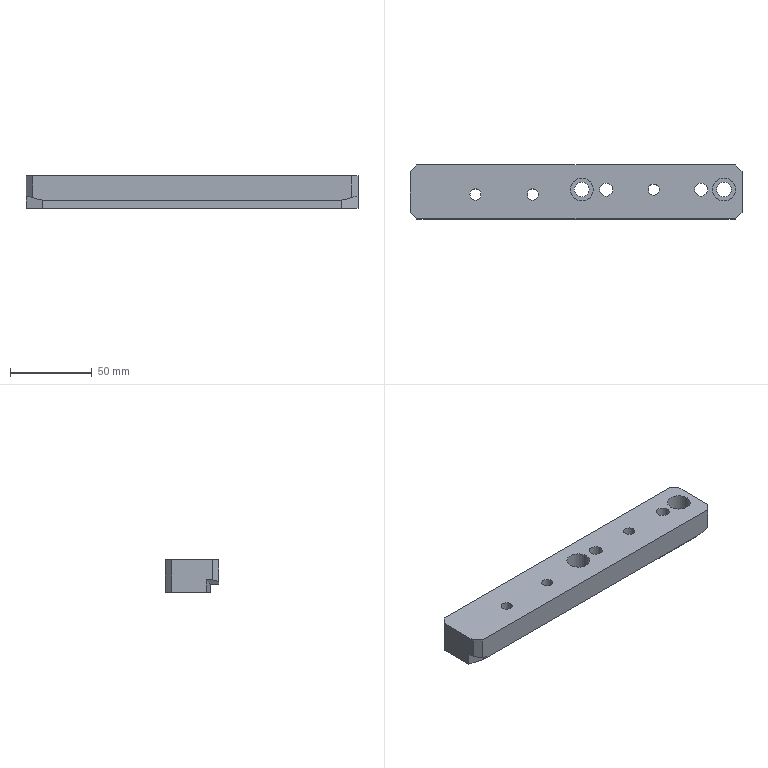Part | NX | features 20 2 | 1 solid | 27 faces | box 203 x 33 x 20 mm | volume 119525 mm3 | plane 18 | cylinder 9 | commonest cylinder face diameters 6.8 x3 8.001 x2 9 x2 14 x2
STEP:
#1=CARTESIAN_POINT('',(-35.998,435.5,16.5));
#2=VERTEX_POINT('',#1);
#3=CARTESIAN_POINT('',(-39.999,435.5,16.5));
#4=DIRECTION('',(0.,0.,1.));
#5=DIRECTION('',(1.,0.,0.));
#6=AXIS2_PLACEMENT_3D('',#3,#4,#5);
#7=CIRCLE('',#6,4.);
#8=EDGE_CURVE('',#2,#2,#7,.T.);
#9=ORIENTED_EDGE('',*,*,#8,.F.);
#10=EDGE_LOOP('',(#9));
#11=FACE_BOUND('',#10,.T.);
#12=CARTESIAN_POINT('',(22.002,435.5,16.5));
#13=VERTEX_POINT('',#12);
#14=CARTESIAN_POINT('',(18.001,435.5,16.5));
#15=DIRECTION('',(0.,0.,-1.));
#16=DIRECTION('',(1.,0.,0.));
#17=AXIS2_PLACEMENT_3D('',#14,#15,#16);
#18=CIRCLE('',#17,4.);
#19=EDGE_CURVE('',#13,#13,#18,.T.);
#20=ORIENTED_EDGE('',*,*,#19,.T.);
#21=EDGE_LOOP('',(#20));
#22=FACE_BOUND('',#21,.T.);
#23=CARTESIAN_POINT('',(39.001,435.5,16.5));
#24=VERTEX_POINT('',#23);
#25=CARTESIAN_POINT('',(32.001,435.5,16.5));
#26=DIRECTION('',(0.,0.,1.));
#27=DIRECTION('',(1.,0.,0.));
#28=AXIS2_PLACEMENT_3D('',#25,#26,#27);
#29=CIRCLE('',#28,7.);
#30=EDGE_CURVE('',#24,#24,#29,.T.);
#31=ORIENTED_EDGE('',*,*,#30,.F.);
#32=EDGE_LOOP('',(#31));
#33=FACE_BOUND('',#32,.T.);
#34=CARTESIAN_POINT('',(-155.999,417.5,16.5));
#35=VERTEX_POINT('',#34);
#36=CARTESIAN_POINT('',(39.001,417.5,16.5));
#37=VERTEX_POINT('',#36);
#38=CARTESIAN_POINT('',(-24.999,417.5,16.5));
#39=DIRECTION('',(1.,0.,0.));
#40=VECTOR('',#39,1000.);
#41=LINE('',#38,#40);
#42=EDGE_CURVE('',#35,#37,#41,.T.);
#43=ORIENTED_EDGE('',*,*,#42,.T.);
#44=CARTESIAN_POINT('',(43.001,421.5,16.5));
#45=VERTEX_POINT('',#44);
#46=CARTESIAN_POINT('',(39.001,417.5,16.5));
#47=DIRECTION('',(0.7071,0.7071,0.));
#48=VECTOR('',#47,1000.);
#49=LINE('',#46,#48);
#50=EDGE_CURVE('',#37,#45,#49,.T.);
#51=ORIENTED_EDGE('',*,*,#50,.T.);
#52=CARTESIAN_POINT('',(43.001,446.5,16.5));
#53=VERTEX_POINT('',#52);
#54=CARTESIAN_POINT('',(43.001,450.5,16.5));
#55=DIRECTION('',(0.,1.,0.));
#56=VECTOR('',#55,1000.);
#57=LINE('',#54,#56);
#58=EDGE_CURVE('',#45,#53,#57,.T.);
#59=ORIENTED_EDGE('',*,*,#58,.T.);
#60=CARTESIAN_POINT('',(39.001,450.5,16.5));
#61=VERTEX_POINT('',#60);
#62=CARTESIAN_POINT('',(43.001,446.5,16.5));
#63=DIRECTION('',(-0.7071,0.7071,0.));
#64=VECTOR('',#63,1000.);
#65=LINE('',#62,#64);
#66=EDGE_CURVE('',#53,#61,#65,.T.);
#67=ORIENTED_EDGE('',*,*,#66,.T.);
#68=CARTESIAN_POINT('',(-155.999,450.5,16.5));
#69=VERTEX_POINT('',#68);
#70=CARTESIAN_POINT('',(-104.999,450.5,16.5));
#71=DIRECTION('',(-1.,0.,0.));
#72=VECTOR('',#71,1000.);
#73=LINE('',#70,#72);
#74=EDGE_CURVE('',#61,#69,#73,.T.);
#75=ORIENTED_EDGE('',*,*,#74,.T.);
#76=CARTESIAN_POINT('',(-159.999,446.5,16.5));
#77=VERTEX_POINT('',#76);
#78=CARTESIAN_POINT('',(-155.999,450.5,16.5));
#79=DIRECTION('',(-0.7071,-0.7071,0.));
#80=VECTOR('',#79,1000.);
#81=LINE('',#78,#80);
#82=EDGE_CURVE('',#69,#77,#81,.T.);
#83=ORIENTED_EDGE('',*,*,#82,.T.);
#84=CARTESIAN_POINT('',(-159.999,421.5,16.5));
#85=VERTEX_POINT('',#84);
#86=CARTESIAN_POINT('',(-159.999,417.5,16.5));
#87=DIRECTION('',(0.,-1.,0.));
#88=VECTOR('',#87,1000.);
#89=LINE('',#86,#88);
#90=EDGE_CURVE('',#77,#85,#89,.T.);
#91=ORIENTED_EDGE('',*,*,#90,.T.);
#92=CARTESIAN_POINT('',(-159.999,421.5,16.5));
#93=DIRECTION('',(0.7071,-0.7071,0.));
#94=VECTOR('',#93,1000.);
#95=LINE('',#92,#94);
#96=EDGE_CURVE('',#85,#35,#95,.T.);
#97=ORIENTED_EDGE('',*,*,#96,.T.);
#98=EDGE_LOOP('',(#43,#51,#59,#67,#75,#83,#91,#97));
#99=FACE_BOUND('',#98,.T.);
#100=CARTESIAN_POINT('',(-81.599,432.45,16.5));
#101=VERTEX_POINT('',#100);
#102=CARTESIAN_POINT('',(-84.999,432.45,16.5));
#103=DIRECTION('',(0.,0.,1.));
#104=DIRECTION('',(1.,0.,0.));
#105=AXIS2_PLACEMENT_3D('',#102,#103,#104);
#106=CIRCLE('',#105,3.4);
#107=EDGE_CURVE('',#101,#101,#106,.T.);
#108=ORIENTED_EDGE('',*,*,#107,.F.);
#109=EDGE_LOOP('',(#108));
#110=FACE_BOUND('',#109,.T.);
#111=CARTESIAN_POINT('',(-116.599,432.45,16.5));
#112=VERTEX_POINT('',#111);
#113=CARTESIAN_POINT('',(-119.999,432.45,16.5));
#114=DIRECTION('',(0.,0.,1.));
#115=DIRECTION('',(1.,0.,0.));
#116=AXIS2_PLACEMENT_3D('',#113,#114,#115);
#117=CIRCLE('',#116,3.4);
#118=EDGE_CURVE('',#112,#112,#117,.T.);
#119=ORIENTED_EDGE('',*,*,#118,.F.);
#120=EDGE_LOOP('',(#119));
#121=FACE_BOUND('',#120,.T.);
#122=CARTESIAN_POINT('',(-47.999,435.5,16.5));
#123=VERTEX_POINT('',#122);
#124=CARTESIAN_POINT('',(-54.999,435.5,16.5));
#125=DIRECTION('',(0.,0.,1.));
#126=DIRECTION('',(1.,0.,0.));
#127=AXIS2_PLACEMENT_3D('',#124,#125,#126);
#128=CIRCLE('',#127,7.);
#129=EDGE_CURVE('',#123,#123,#128,.T.);
#130=ORIENTED_EDGE('',*,*,#129,.F.);
#131=EDGE_LOOP('',(#130));
#132=FACE_BOUND('',#131,.T.);
#133=CARTESIAN_POINT('',(-7.599,435.5,16.5));
#134=VERTEX_POINT('',#133);
#135=CARTESIAN_POINT('',(-10.999,435.5,16.5));
#136=DIRECTION('',(0.,0.,-1.));
#137=DIRECTION('',(1.,0.,0.));
#138=AXIS2_PLACEMENT_3D('',#135,#136,#137);
#139=CIRCLE('',#138,3.4);
#140=EDGE_CURVE('',#134,#134,#139,.T.);
#141=ORIENTED_EDGE('',*,*,#140,.T.);
#142=EDGE_LOOP('',(#141));
#143=FACE_BOUND('',#142,.T.);
#144=CARTESIAN_POINT('',(-24.999,450.5,16.5));
#145=DIRECTION('',(0.,0.,1.));
#146=DIRECTION('',(-1.,0.,0.));
#147=AXIS2_PLACEMENT_3D('',#144,#145,#146);
#148=PLANE('',#147);
#149=ADVANCED_FACE('',(#11,#22,#33,#99,#110,#121,#132,#143),#148,.T.);
#150=CARTESIAN_POINT('',(-35.998,435.5,-3.5));
#151=VERTEX_POINT('',#150);
#152=CARTESIAN_POINT('',(-39.999,435.5,-3.5));
#153=DIRECTION('',(0.,0.,1.));
#154=DIRECTION('',(1.,0.,0.));
#155=AXIS2_PLACEMENT_3D('',#152,#153,#154);
#156=CIRCLE('',#155,4.);
#157=EDGE_CURVE('',#151,#151,#156,.T.);
#158=ORIENTED_EDGE('',*,*,#157,.F.);
#159=EDGE_LOOP('',(#158));
#160=FACE_BOUND('',#159,.T.);
#161=ORIENTED_EDGE('',*,*,#8,.T.);
#162=EDGE_LOOP('',(#161));
#163=FACE_BOUND('',#162,.T.);
#164=CARTESIAN_POINT('',(-39.999,435.5,42.5));
#165=DIRECTION('',(0.,0.,-1.));
#166=DIRECTION('',(1.,0.,0.));
#167=AXIS2_PLACEMENT_3D('',#164,#165,#166);
#168=CYLINDRICAL_SURFACE('',#167,4.);
#169=ADVANCED_FACE('',(#160,#163),#168,.F.);
#170=CARTESIAN_POINT('',(22.002,435.5,-3.5));
#171=VERTEX_POINT('',#170);
#172=CARTESIAN_POINT('',(18.001,435.5,-3.5));
#173=DIRECTION('',(0.,0.,-1.));
#174=DIRECTION('',(1.,0.,0.));
#175=AXIS2_PLACEMENT_3D('',#172,#173,#174);
#176=CIRCLE('',#175,4.);
#177=EDGE_CURVE('',#171,#171,#176,.T.);
#178=ORIENTED_EDGE('',*,*,#177,.T.);
#179=EDGE_LOOP('',(#178));
#180=FACE_BOUND('',#179,.T.);
#181=ORIENTED_EDGE('',*,*,#19,.F.);
#182=EDGE_LOOP('',(#181));
#183=FACE_BOUND('',#182,.T.);
#184=CARTESIAN_POINT('',(18.001,435.5,42.5));
#185=DIRECTION('',(0.,0.,-1.));
#186=DIRECTION('',(1.,0.,0.));
#187=AXIS2_PLACEMENT_3D('',#184,#185,#186);
#188=CYLINDRICAL_SURFACE('',#187,4.);
#189=ADVANCED_FACE('',(#180,#183),#188,.F.);
#190=CARTESIAN_POINT('',(36.501,435.5,6.5));
#191=VERTEX_POINT('',#190);
#192=CARTESIAN_POINT('',(32.001,435.5,6.5));
#193=DIRECTION('',(0.,0.,-1.));
#194=DIRECTION('',(1.,0.,0.));
#195=AXIS2_PLACEMENT_3D('',#192,#193,#194);
#196=CIRCLE('',#195,4.5);
#197=EDGE_CURVE('',#191,#191,#196,.T.);
#198=ORIENTED_EDGE('',*,*,#197,.T.);
#199=EDGE_LOOP('',(#198));
#200=FACE_BOUND('',#199,.T.);
#201=CARTESIAN_POINT('',(39.001,435.5,6.5));
#202=VERTEX_POINT('',#201);
#203=CARTESIAN_POINT('',(32.001,435.5,6.5));
#204=DIRECTION('',(0.,0.,1.));
#205=DIRECTION('',(1.,0.,0.));
#206=AXIS2_PLACEMENT_3D('',#203,#204,#205);
#207=CIRCLE('',#206,7.);
#208=EDGE_CURVE('',#202,#202,#207,.T.);
#209=ORIENTED_EDGE('',*,*,#208,.T.);
#210=EDGE_LOOP('',(#209));
#211=FACE_BOUND('',#210,.T.);
#212=CARTESIAN_POINT('',(265.844,302.3,6.5));
#213=DIRECTION('',(0.,0.,1.));
#214=DIRECTION('',(0.,1.,0.));
#215=AXIS2_PLACEMENT_3D('',#212,#213,#214);
#216=PLANE('',#215);
#217=ADVANCED_FACE('',(#200,#211),#216,.T.);
#218=CARTESIAN_POINT('',(-159.999,425.179,4.179));
#219=VERTEX_POINT('',#218);
#220=CARTESIAN_POINT('',(-159.999,421.5,4.179));
#221=VERTEX_POINT('',#220);
#222=CARTESIAN_POINT('',(-159.999,425.179,4.179));
#223=DIRECTION('',(0.,-1.,0.));
#224=VECTOR('',#223,1000.);
#225=LINE('',#222,#224);
#226=EDGE_CURVE('',#219,#221,#225,.T.);
#227=ORIENTED_EDGE('',*,*,#226,.F.);
#228=CARTESIAN_POINT('',(-150.,422.5,1.5));
#229=VERTEX_POINT('',#228);
#230=CARTESIAN_POINT('',(-150.,422.5,1.5));
#231=DIRECTION('',(-0.9351,0.2506,0.2506));
#232=VECTOR('',#231,1000.);
#233=LINE('',#230,#232);
#234=EDGE_CURVE('',#229,#219,#233,.T.);
#235=ORIENTED_EDGE('',*,*,#234,.F.);
#236=CARTESIAN_POINT('',(-149.999,422.5,1.5));
#237=VERTEX_POINT('',#236);
#238=CARTESIAN_POINT('',(-94.02,422.5,-13.5));
#239=DIRECTION('',(-0.9659,0.,0.2588));
#240=VECTOR('',#239,1000.);
#241=LINE('',#238,#240);
#242=EDGE_CURVE('',#237,#229,#241,.T.);
#243=ORIENTED_EDGE('',*,*,#242,.F.);
#244=CARTESIAN_POINT('',(-149.999,417.5,1.5));
#245=VERTEX_POINT('',#244);
#246=CARTESIAN_POINT('',(-149.999,417.5,1.5));
#247=DIRECTION('',(0.,1.,0.));
#248=VECTOR('',#247,1000.);
#249=LINE('',#246,#248);
#250=EDGE_CURVE('',#245,#237,#249,.T.);
#251=ORIENTED_EDGE('',*,*,#250,.F.);
#252=CARTESIAN_POINT('',(-155.999,417.5,3.108));
#253=VERTEX_POINT('',#252);
#254=CARTESIAN_POINT('',(-149.999,417.5,1.5));
#255=DIRECTION('',(0.9659,0.,-0.2588));
#256=VECTOR('',#255,1000.);
#257=LINE('',#254,#256);
#258=EDGE_CURVE('',#253,#245,#257,.T.);
#259=ORIENTED_EDGE('',*,*,#258,.F.);
#260=CARTESIAN_POINT('',(-142.948,404.449,-0.3894));
#261=DIRECTION('',(-0.6947,0.6947,0.1862));
#262=VECTOR('',#261,1000.);
#263=LINE('',#260,#262);
#264=EDGE_CURVE('',#253,#221,#263,.T.);
#265=ORIENTED_EDGE('',*,*,#264,.T.);
#266=EDGE_LOOP('',(#227,#235,#243,#251,#259,#265));
#267=FACE_BOUND('',#266,.T.);
#268=CARTESIAN_POINT('',(-149.999,396.891,1.5));
#269=DIRECTION('',(-0.2588,0.,-0.9659));
#270=DIRECTION('',(0.9659,0.,-0.2588));
#271=AXIS2_PLACEMENT_3D('',#268,#269,#270);
#272=PLANE('',#271);
#273=ADVANCED_FACE('',(#267),#272,.T.);
#274=ORIENTED_EDGE('',*,*,#250,.T.);
#275=CARTESIAN_POINT('',(32.999,422.5,1.5));
#276=VERTEX_POINT('',#275);
#277=CARTESIAN_POINT('',(-35.001,422.5,1.5));
#278=DIRECTION('',(-1.,0.,0.));
#279=VECTOR('',#278,1000.);
#280=LINE('',#277,#279);
#281=EDGE_CURVE('',#276,#237,#280,.T.);
#282=ORIENTED_EDGE('',*,*,#281,.F.);
#283=CARTESIAN_POINT('',(33.001,422.5,1.5));
#284=VERTEX_POINT('',#283);
#285=CARTESIAN_POINT('',(43.001,425.18,1.5));
#286=DIRECTION('',(-0.9659,-0.2588,0.));
#287=VECTOR('',#286,1000.);
#288=LINE('',#285,#287);
#289=EDGE_CURVE('',#284,#276,#288,.T.);
#290=ORIENTED_EDGE('',*,*,#289,.F.);
#291=CARTESIAN_POINT('',(33.001,417.5,1.5));
#292=VERTEX_POINT('',#291);
#293=CARTESIAN_POINT('',(33.001,425.18,1.5));
#294=DIRECTION('',(0.,-1.,0.));
#295=VECTOR('',#294,1000.);
#296=LINE('',#293,#295);
#297=EDGE_CURVE('',#284,#292,#296,.T.);
#298=ORIENTED_EDGE('',*,*,#297,.T.);
#299=CARTESIAN_POINT('',(-24.999,417.5,1.5));
#300=DIRECTION('',(-1.,0.,0.));
#301=VECTOR('',#300,1000.);
#302=LINE('',#299,#301);
#303=EDGE_CURVE('',#292,#245,#302,.T.);
#304=ORIENTED_EDGE('',*,*,#303,.T.);
#305=EDGE_LOOP('',(#274,#282,#290,#298,#304));
#306=FACE_BOUND('',#305,.T.);
#307=CARTESIAN_POINT('',(-2.728,396.891,1.5));
#308=DIRECTION('',(0.,0.,-1.));
#309=DIRECTION('',(1.,0.,0.));
#310=AXIS2_PLACEMENT_3D('',#307,#308,#309);
#311=PLANE('',#310);
#312=ADVANCED_FACE('',(#306),#311,.T.);
#313=CARTESIAN_POINT('',(39.001,417.5,3.108));
#314=VERTEX_POINT('',#313);
#315=CARTESIAN_POINT('',(33.001,417.5,1.5));
#316=DIRECTION('',(0.9659,0.,0.2588));
#317=VECTOR('',#316,1000.);
#318=LINE('',#315,#317);
#319=EDGE_CURVE('',#292,#314,#318,.T.);
#320=ORIENTED_EDGE('',*,*,#319,.F.);
#321=ORIENTED_EDGE('',*,*,#297,.F.);
#322=CARTESIAN_POINT('',(43.001,425.18,4.179));
#323=VERTEX_POINT('',#322);
#324=CARTESIAN_POINT('',(42.373,425.012,4.011));
#325=DIRECTION('',(-0.9351,-0.2506,-0.2506));
#326=VECTOR('',#325,1000.);
#327=LINE('',#324,#326);
#328=EDGE_CURVE('',#323,#284,#327,.T.);
#329=ORIENTED_EDGE('',*,*,#328,.F.);
#330=CARTESIAN_POINT('',(43.001,421.5,4.179));
#331=VERTEX_POINT('',#330);
#332=CARTESIAN_POINT('',(43.001,417.5,4.179));
#333=DIRECTION('',(0.,1.,0.));
#334=VECTOR('',#333,1000.);
#335=LINE('',#332,#334);
#336=EDGE_CURVE('',#331,#323,#335,.T.);
#337=ORIENTED_EDGE('',*,*,#336,.F.);
#338=CARTESIAN_POINT('',(25.95,404.449,-0.3894));
#339=DIRECTION('',(-0.6947,-0.6947,-0.1862));
#340=VECTOR('',#339,1000.);
#341=LINE('',#338,#340);
#342=EDGE_CURVE('',#331,#314,#341,.T.);
#343=ORIENTED_EDGE('',*,*,#342,.T.);
#344=EDGE_LOOP('',(#320,#321,#329,#337,#343));
#345=FACE_BOUND('',#344,.T.);
#346=CARTESIAN_POINT('',(33.001,396.891,1.5));
#347=DIRECTION('',(0.2588,0.,-0.9659));
#348=DIRECTION('',(0.9659,0.,0.2588));
#349=AXIS2_PLACEMENT_3D('',#346,#347,#348);
#350=PLANE('',#349);
#351=ADVANCED_FACE('',(#345),#350,.T.);
#352=ORIENTED_EDGE('',*,*,#30,.T.);
#353=EDGE_LOOP('',(#352));
#354=FACE_BOUND('',#353,.T.);
#355=ORIENTED_EDGE('',*,*,#208,.F.);
#356=EDGE_LOOP('',(#355));
#357=FACE_BOUND('',#356,.T.);
#358=CARTESIAN_POINT('',(32.001,435.5,42.5));
#359=DIRECTION('',(0.,0.,-1.));
#360=DIRECTION('',(1.,0.,0.));
#361=AXIS2_PLACEMENT_3D('',#358,#359,#360);
#362=CYLINDRICAL_SURFACE('',#361,7.);
#363=ADVANCED_FACE('',(#354,#357),#362,.F.);
#364=ORIENTED_EDGE('',*,*,#96,.F.);
#365=CARTESIAN_POINT('',(-159.999,421.5,11.5));
#366=DIRECTION('',(0.,0.,1.));
#367=VECTOR('',#366,1000.);
#368=LINE('',#365,#367);
#369=EDGE_CURVE('',#221,#85,#368,.T.);
#370=ORIENTED_EDGE('',*,*,#369,.F.);
#371=ORIENTED_EDGE('',*,*,#264,.F.);
#372=CARTESIAN_POINT('',(-155.999,417.5,11.5));
#373=DIRECTION('',(0.,0.,-1.));
#374=VECTOR('',#373,1000.);
#375=LINE('',#372,#374);
#376=EDGE_CURVE('',#35,#253,#375,.T.);
#377=ORIENTED_EDGE('',*,*,#376,.F.);
#378=EDGE_LOOP('',(#364,#370,#371,#377));
#379=FACE_BOUND('',#378,.T.);
#380=CARTESIAN_POINT('',(-159.999,421.5,11.5));
#381=DIRECTION('',(0.7071,0.7071,0.));
#382=DIRECTION('',(0.,0.,-1.));
#383=AXIS2_PLACEMENT_3D('',#380,#381,#382);
#384=PLANE('',#383);
#385=ADVANCED_FACE('',(#379),#384,.F.);
#386=ORIENTED_EDGE('',*,*,#50,.F.);
#387=CARTESIAN_POINT('',(39.001,417.5,11.5));
#388=DIRECTION('',(0.,0.,1.));
#389=VECTOR('',#388,1000.);
#390=LINE('',#387,#389);
#391=EDGE_CURVE('',#314,#37,#390,.T.);
#392=ORIENTED_EDGE('',*,*,#391,.F.);
#393=ORIENTED_EDGE('',*,*,#342,.F.);
#394=CARTESIAN_POINT('',(43.001,421.5,11.5));
#395=DIRECTION('',(0.,0.,-1.));
#396=VECTOR('',#395,1000.);
#397=LINE('',#394,#396);
#398=EDGE_CURVE('',#45,#331,#397,.T.);
#399=ORIENTED_EDGE('',*,*,#398,.F.);
#400=EDGE_LOOP('',(#386,#392,#393,#399));
#401=FACE_BOUND('',#400,.T.);
#402=CARTESIAN_POINT('',(39.001,417.5,11.5));
#403=DIRECTION('',(-0.7071,0.7071,0.));
#404=DIRECTION('',(0.,0.,-1.));
#405=AXIS2_PLACEMENT_3D('',#402,#403,#404);
#406=PLANE('',#405);
#407=ADVANCED_FACE('',(#401),#406,.F.);
#408=ORIENTED_EDGE('',*,*,#258,.T.);
#409=ORIENTED_EDGE('',*,*,#303,.F.);
#410=ORIENTED_EDGE('',*,*,#319,.T.);
#411=ORIENTED_EDGE('',*,*,#391,.T.);
#412=ORIENTED_EDGE('',*,*,#42,.F.);
#413=ORIENTED_EDGE('',*,*,#376,.T.);
#414=EDGE_LOOP('',(#408,#409,#410,#411,#412,#413));
#415=FACE_BOUND('',#414,.T.);
#416=CARTESIAN_POINT('',(-24.999,417.5,11.5));
#417=DIRECTION('',(0.,1.,0.));
#418=DIRECTION('',(0.,0.,1.));
#419=AXIS2_PLACEMENT_3D('',#416,#417,#418);
#420=PLANE('',#419);
#421=ADVANCED_FACE('',(#415),#420,.F.);
#422=ORIENTED_EDGE('',*,*,#197,.F.);
#423=EDGE_LOOP('',(#422));
#424=FACE_BOUND('',#423,.T.);
#425=CARTESIAN_POINT('',(36.501,435.5,-3.5));
#426=VERTEX_POINT('',#425);
#427=CARTESIAN_POINT('',(32.001,435.5,-3.5));
#428=DIRECTION('',(0.,0.,1.));
#429=DIRECTION('',(1.,0.,0.));
#430=AXIS2_PLACEMENT_3D('',#427,#428,#429);
#431=CIRCLE('',#430,4.5);
#432=EDGE_CURVE('',#426,#426,#431,.T.);
#433=ORIENTED_EDGE('',*,*,#432,.F.);
#434=EDGE_LOOP('',(#433));
#435=FACE_BOUND('',#434,.T.);
#436=CARTESIAN_POINT('',(32.001,435.5,42.5));
#437=DIRECTION('',(0.,0.,-1.));
#438=DIRECTION('',(1.,0.,0.));
#439=AXIS2_PLACEMENT_3D('',#436,#437,#438);
#440=CYLINDRICAL_SURFACE('',#439,4.5);
#441=ADVANCED_FACE('',(#424,#435),#440,.F.);
#442=ORIENTED_EDGE('',*,*,#58,.F.);
#443=ORIENTED_EDGE('',*,*,#398,.T.);
#444=ORIENTED_EDGE('',*,*,#336,.T.);
#445=CARTESIAN_POINT('',(43.001,425.18,-3.5));
#446=VERTEX_POINT('',#445);
#447=CARTESIAN_POINT('',(43.001,425.18,3.5));
#448=DIRECTION('',(0.,0.,1.));
#449=VECTOR('',#448,1000.);
#450=LINE('',#447,#449);
#451=EDGE_CURVE('',#446,#323,#450,.T.);
#452=ORIENTED_EDGE('',*,*,#451,.F.);
#453=CARTESIAN_POINT('',(43.001,446.5,-3.5));
#454=VERTEX_POINT('',#453);
#455=CARTESIAN_POINT('',(43.001,450.5,-3.5));
#456=DIRECTION('',(0.,1.,0.));
#457=VECTOR('',#456,1000.);
#458=LINE('',#455,#457);
#459=EDGE_CURVE('',#446,#454,#458,.T.);
#460=ORIENTED_EDGE('',*,*,#459,.T.);
#461=CARTESIAN_POINT('',(43.001,446.5,11.5));
#462=DIRECTION('',(0.,0.,1.));
#463=VECTOR('',#462,1000.);
#464=LINE('',#461,#463);
#465=EDGE_CURVE('',#454,#53,#464,.T.);
#466=ORIENTED_EDGE('',*,*,#465,.T.);
#467=EDGE_LOOP('',(#442,#443,#444,#452,#460,#466));
#468=FACE_BOUND('',#467,.T.);
#469=CARTESIAN_POINT('',(43.001,450.5,11.5));
#470=DIRECTION('',(-1.,0.,0.));
#471=DIRECTION('',(0.,0.,-1.));
#472=AXIS2_PLACEMENT_3D('',#469,#470,#471);
#473=PLANE('',#472);
#474=ADVANCED_FACE('',(#468),#473,.F.);
#475=ORIENTED_EDGE('',*,*,#66,.F.);
#476=ORIENTED_EDGE('',*,*,#465,.F.);
#477=CARTESIAN_POINT('',(39.001,450.5,-3.5));
#478=VERTEX_POINT('',#477);
#479=CARTESIAN_POINT('',(43.001,446.5,-3.5));
#480=DIRECTION('',(0.7071,-0.7071,0.));
#481=VECTOR('',#480,1000.);
#482=LINE('',#479,#481);
#483=EDGE_CURVE('',#478,#454,#482,.T.);
#484=ORIENTED_EDGE('',*,*,#483,.F.);
#485=CARTESIAN_POINT('',(39.001,450.5,11.5));
#486=DIRECTION('',(0.,0.,-1.));
#487=VECTOR('',#486,1000.);
#488=LINE('',#485,#487);
#489=EDGE_CURVE('',#61,#478,#488,.T.);
#490=ORIENTED_EDGE('',*,*,#489,.F.);
#491=EDGE_LOOP('',(#475,#476,#484,#490));
#492=FACE_BOUND('',#491,.T.);
#493=CARTESIAN_POINT('',(43.001,446.5,11.5));
#494=DIRECTION('',(-0.7071,-0.7071,0.));
#495=DIRECTION('',(0.,0.,-1.));
#496=AXIS2_PLACEMENT_3D('',#493,#494,#495);
#497=PLANE('',#496);
#498=ADVANCED_FACE('',(#492),#497,.F.);
#499=CARTESIAN_POINT('',(-155.999,450.5,-3.5));
#500=VERTEX_POINT('',#499);
#501=CARTESIAN_POINT('',(-104.999,450.5,-3.5));
#502=DIRECTION('',(-1.,0.,0.));
#503=VECTOR('',#502,1000.);
#504=LINE('',#501,#503);
#505=EDGE_CURVE('',#478,#500,#504,.T.);
#506=ORIENTED_EDGE('',*,*,#505,.T.);
#507=CARTESIAN_POINT('',(-155.999,450.5,11.5));
#508=DIRECTION('',(0.,0.,1.));
#509=VECTOR('',#508,1000.);
#510=LINE('',#507,#509);
#511=EDGE_CURVE('',#500,#69,#510,.T.);
#512=ORIENTED_EDGE('',*,*,#511,.T.);
#513=ORIENTED_EDGE('',*,*,#74,.F.);
#514=ORIENTED_EDGE('',*,*,#489,.T.);
#515=EDGE_LOOP('',(#506,#512,#513,#514));
#516=FACE_BOUND('',#515,.T.);
#517=CARTESIAN_POINT('',(-104.999,450.5,11.5));
#518=DIRECTION('',(0.,-1.,0.));
#519=DIRECTION('',(0.,0.,-1.));
#520=AXIS2_PLACEMENT_3D('',#517,#518,#519);
#521=PLANE('',#520);
#522=ADVANCED_FACE('',(#516),#521,.F.);
#523=ORIENTED_EDGE('',*,*,#82,.F.);
#524=ORIENTED_EDGE('',*,*,#511,.F.);
#525=CARTESIAN_POINT('',(-159.999,446.5,-3.5));
#526=VERTEX_POINT('',#525);
#527=CARTESIAN_POINT('',(-155.999,450.5,-3.5));
#528=DIRECTION('',(0.7071,0.7071,0.));
#529=VECTOR('',#528,1000.);
#530=LINE('',#527,#529);
#531=EDGE_CURVE('',#526,#500,#530,.T.);
#532=ORIENTED_EDGE('',*,*,#531,.F.);
#533=CARTESIAN_POINT('',(-159.999,446.5,11.5));
#534=DIRECTION('',(0.,0.,-1.));
#535=VECTOR('',#534,1000.);
#536=LINE('',#533,#535);
#537=EDGE_CURVE('',#77,#526,#536,.T.);
#538=ORIENTED_EDGE('',*,*,#537,.F.);
#539=EDGE_LOOP('',(#523,#524,#532,#538));
#540=FACE_BOUND('',#539,.T.);
#541=CARTESIAN_POINT('',(-155.999,450.5,11.5));
#542=DIRECTION('',(0.7071,-0.7071,0.));
#543=DIRECTION('',(0.,0.,-1.));
#544=AXIS2_PLACEMENT_3D('',#541,#542,#543);
#545=PLANE('',#544);
#546=ADVANCED_FACE('',(#540),#545,.F.);
#547=CARTESIAN_POINT('',(-159.999,425.179,-3.5));
#548=VERTEX_POINT('',#547);
#549=CARTESIAN_POINT('',(-159.999,417.5,-3.5));
#550=DIRECTION('',(0.,-1.,0.));
#551=VECTOR('',#550,1000.);
#552=LINE('',#549,#551);
#553=EDGE_CURVE('',#526,#548,#552,.T.);
#554=ORIENTED_EDGE('',*,*,#553,.T.);
#555=CARTESIAN_POINT('',(-159.999,425.179,3.5));
#556=DIRECTION('',(0.,0.,1.));
#557=VECTOR('',#556,1000.);
#558=LINE('',#555,#557);
#559=EDGE_CURVE('',#548,#219,#558,.T.);
#560=ORIENTED_EDGE('',*,*,#559,.T.);
#561=ORIENTED_EDGE('',*,*,#226,.T.);
#562=ORIENTED_EDGE('',*,*,#369,.T.);
#563=ORIENTED_EDGE('',*,*,#90,.F.);
#564=ORIENTED_EDGE('',*,*,#537,.T.);
#565=EDGE_LOOP('',(#554,#560,#561,#562,#563,#564));
#566=FACE_BOUND('',#565,.T.);
#567=CARTESIAN_POINT('',(-159.999,417.5,11.5));
#568=DIRECTION('',(1.,0.,0.));
#569=DIRECTION('',(0.,0.,1.));
#570=AXIS2_PLACEMENT_3D('',#567,#568,#569);
#571=PLANE('',#570);
#572=ADVANCED_FACE('',(#566),#571,.F.);
#573=CARTESIAN_POINT('',(-150.,422.5,-3.5));
#574=VERTEX_POINT('',#573);
#575=CARTESIAN_POINT('',(-150.,422.5,-3.5));
#576=DIRECTION('',(0.9659,-0.2588,0.));
#577=VECTOR('',#576,1000.);
#578=LINE('',#575,#577);
#579=EDGE_CURVE('',#548,#574,#578,.T.);
#580=ORIENTED_EDGE('',*,*,#579,.T.);
#581=CARTESIAN_POINT('',(-150.,422.5,3.5));
#582=DIRECTION('',(0.,0.,-1.));
#583=VECTOR('',#582,1000.);
#584=LINE('',#581,#583);
#585=EDGE_CURVE('',#229,#574,#584,.T.);
#586=ORIENTED_EDGE('',*,*,#585,.F.);
#587=ORIENTED_EDGE('',*,*,#234,.T.);
#588=ORIENTED_EDGE('',*,*,#559,.F.);
#589=EDGE_LOOP('',(#580,#586,#587,#588));
#590=FACE_BOUND('',#589,.T.);
#591=CARTESIAN_POINT('',(-150.,422.5,3.5));
#592=DIRECTION('',(0.2588,0.9659,0.));
#593=DIRECTION('',(0.9659,-0.2588,0.));
#594=AXIS2_PLACEMENT_3D('',#591,#592,#593);
#595=PLANE('',#594);
#596=ADVANCED_FACE('',(#590),#595,.F.);
#597=CARTESIAN_POINT('',(32.999,422.5,-3.5));
#598=VERTEX_POINT('',#597);
#599=CARTESIAN_POINT('',(-35.001,422.5,-3.5));
#600=DIRECTION('',(1.,0.,0.));
#601=VECTOR('',#600,1000.);
#602=LINE('',#599,#601);
#603=EDGE_CURVE('',#574,#598,#602,.T.);
#604=ORIENTED_EDGE('',*,*,#603,.T.);
#605=CARTESIAN_POINT('',(32.999,422.5,3.5));
#606=DIRECTION('',(0.,0.,-1.));
#607=VECTOR('',#606,1000.);
#608=LINE('',#605,#607);
#609=EDGE_CURVE('',#276,#598,#608,.T.);
#610=ORIENTED_EDGE('',*,*,#609,.F.);
#611=ORIENTED_EDGE('',*,*,#281,.T.);
#612=ORIENTED_EDGE('',*,*,#242,.T.);
#613=ORIENTED_EDGE('',*,*,#585,.T.);
#614=EDGE_LOOP('',(#604,#610,#611,#612,#613));
#615=FACE_BOUND('',#614,.T.);
#616=CARTESIAN_POINT('',(-35.001,422.5,3.5));
#617=DIRECTION('',(0.,1.,0.));
#618=DIRECTION('',(0.,0.,1.));
#619=AXIS2_PLACEMENT_3D('',#616,#617,#618);
#620=PLANE('',#619);
#621=ADVANCED_FACE('',(#615),#620,.F.);
#622=CARTESIAN_POINT('',(43.001,425.18,-3.5));
#623=DIRECTION('',(0.9659,0.2588,0.));
#624=VECTOR('',#623,1000.);
#625=LINE('',#622,#624);
#626=EDGE_CURVE('',#598,#446,#625,.T.);
#627=ORIENTED_EDGE('',*,*,#626,.T.);
#628=ORIENTED_EDGE('',*,*,#451,.T.);
#629=ORIENTED_EDGE('',*,*,#328,.T.);
#630=ORIENTED_EDGE('',*,*,#289,.T.);
#631=ORIENTED_EDGE('',*,*,#609,.T.);
#632=EDGE_LOOP('',(#627,#628,#629,#630,#631));
#633=FACE_BOUND('',#632,.T.);
#634=CARTESIAN_POINT('',(43.001,425.18,3.5));
#635=DIRECTION('',(-0.2588,0.9659,0.));
#636=DIRECTION('',(0.9659,0.2588,0.));
#637=AXIS2_PLACEMENT_3D('',#634,#635,#636);
#638=PLANE('',#637);
#639=ADVANCED_FACE('',(#633),#638,.F.);
#640=ORIENTED_EDGE('',*,*,#107,.T.);
#641=EDGE_LOOP('',(#640));
#642=FACE_BOUND('',#641,.T.);
#643=CARTESIAN_POINT('',(-81.599,432.45,-3.5));
#644=VERTEX_POINT('',#643);
#645=CARTESIAN_POINT('',(-84.999,432.45,-3.5));
#646=DIRECTION('',(0.,0.,1.));
#647=DIRECTION('',(1.,0.,0.));
#648=AXIS2_PLACEMENT_3D('',#645,#646,#647);
#649=CIRCLE('',#648,3.4);
#650=EDGE_CURVE('',#644,#644,#649,.T.);
#651=ORIENTED_EDGE('',*,*,#650,.F.);
#652=EDGE_LOOP('',(#651));
#653=FACE_BOUND('',#652,.T.);
#654=CARTESIAN_POINT('',(-84.999,432.45,-3.5));
#655=DIRECTION('',(0.,0.,1.));
#656=DIRECTION('',(1.,0.,0.));
#657=AXIS2_PLACEMENT_3D('',#654,#655,#656);
#658=CYLINDRICAL_SURFACE('',#657,3.4);
#659=ADVANCED_FACE('',(#642,#653),#658,.F.);
#660=ORIENTED_EDGE('',*,*,#118,.T.);
#661=EDGE_LOOP('',(#660));
#662=FACE_BOUND('',#661,.T.);
#663=CARTESIAN_POINT('',(-116.599,432.45,-3.5));
#664=VERTEX_POINT('',#663);
#665=CARTESIAN_POINT('',(-119.999,432.45,-3.5));
#666=DIRECTION('',(0.,0.,1.));
#667=DIRECTION('',(1.,0.,0.));
#668=AXIS2_PLACEMENT_3D('',#665,#666,#667);
#669=CIRCLE('',#668,3.4);
#670=EDGE_CURVE('',#664,#664,#669,.T.);
#671=ORIENTED_EDGE('',*,*,#670,.F.);
#672=EDGE_LOOP('',(#671));
#673=FACE_BOUND('',#672,.T.);
#674=CARTESIAN_POINT('',(-119.999,432.45,-3.5));
#675=DIRECTION('',(0.,0.,1.));
#676=DIRECTION('',(1.,0.,0.));
#677=AXIS2_PLACEMENT_3D('',#674,#675,#676);
#678=CYLINDRICAL_SURFACE('',#677,3.4);
#679=ADVANCED_FACE('',(#662,#673),#678,.F.);
#680=CARTESIAN_POINT('',(-7.599,435.5,-3.5));
#681=VERTEX_POINT('',#680);
#682=CARTESIAN_POINT('',(-10.999,435.5,-3.5));
#683=DIRECTION('',(0.,0.,1.));
#684=DIRECTION('',(1.,0.,0.));
#685=AXIS2_PLACEMENT_3D('',#682,#683,#684);
#686=CIRCLE('',#685,3.4);
#687=EDGE_CURVE('',#681,#681,#686,.T.);
#688=ORIENTED_EDGE('',*,*,#687,.T.);
#689=EDGE_LOOP('',(#688));
#690=FACE_BOUND('',#689,.T.);
#691=CARTESIAN_POINT('',(-50.499,435.5,-3.5));
#692=VERTEX_POINT('',#691);
#693=CARTESIAN_POINT('',(-54.999,435.5,-3.5));
#694=DIRECTION('',(0.,0.,-1.));
#695=DIRECTION('',(1.,0.,0.));
#696=AXIS2_PLACEMENT_3D('',#693,#694,#695);
#697=CIRCLE('',#696,4.5);
#698=EDGE_CURVE('',#692,#692,#697,.T.);
#699=ORIENTED_EDGE('',*,*,#698,.F.);
#700=EDGE_LOOP('',(#699));
#701=FACE_BOUND('',#700,.T.);
#702=ORIENTED_EDGE('',*,*,#670,.T.);
#703=EDGE_LOOP('',(#702));
#704=FACE_BOUND('',#703,.T.);
#705=ORIENTED_EDGE('',*,*,#650,.T.);
#706=EDGE_LOOP('',(#705));
#707=FACE_BOUND('',#706,.T.);
#708=ORIENTED_EDGE('',*,*,#626,.F.);
#709=ORIENTED_EDGE('',*,*,#603,.F.);
#710=ORIENTED_EDGE('',*,*,#579,.F.);
#711=ORIENTED_EDGE('',*,*,#553,.F.);
#712=ORIENTED_EDGE('',*,*,#531,.T.);
#713=ORIENTED_EDGE('',*,*,#505,.F.);
#714=ORIENTED_EDGE('',*,*,#483,.T.);
#715=ORIENTED_EDGE('',*,*,#459,.F.);
#716=EDGE_LOOP('',(#708,#709,#710,#711,#712,#713,#714,#715));
#717=FACE_BOUND('',#716,.T.);
#718=ORIENTED_EDGE('',*,*,#177,.F.);
#719=EDGE_LOOP('',(#718));
#720=FACE_BOUND('',#719,.T.);
#721=ORIENTED_EDGE('',*,*,#432,.T.);
#722=EDGE_LOOP('',(#721));
#723=FACE_BOUND('',#722,.T.);
#724=ORIENTED_EDGE('',*,*,#157,.T.);
#725=EDGE_LOOP('',(#724));
#726=FACE_BOUND('',#725,.T.);
#727=CARTESIAN_POINT('',(-24.999,450.5,-3.5));
#728=DIRECTION('',(0.,0.,1.));
#729=DIRECTION('',(-1.,0.,0.));
#730=AXIS2_PLACEMENT_3D('',#727,#728,#729);
#731=PLANE('',#730);
#732=ADVANCED_FACE('',(#690,#701,#704,#707,#717,#720,#723,#726),#731,.F.);
#733=CARTESIAN_POINT('',(-50.499,435.5,6.5));
#734=VERTEX_POINT('',#733);
#735=CARTESIAN_POINT('',(-54.999,435.5,6.5));
#736=DIRECTION('',(0.,0.,-1.));
#737=DIRECTION('',(1.,0.,0.));
#738=AXIS2_PLACEMENT_3D('',#735,#736,#737);
#739=CIRCLE('',#738,4.5);
#740=EDGE_CURVE('',#734,#734,#739,.T.);
#741=ORIENTED_EDGE('',*,*,#740,.T.);
#742=EDGE_LOOP('',(#741));
#743=FACE_BOUND('',#742,.T.);
#744=CARTESIAN_POINT('',(-47.999,435.5,6.5));
#745=VERTEX_POINT('',#744);
#746=CARTESIAN_POINT('',(-54.999,435.5,6.5));
#747=DIRECTION('',(0.,0.,1.));
#748=DIRECTION('',(1.,0.,0.));
#749=AXIS2_PLACEMENT_3D('',#746,#747,#748);
#750=CIRCLE('',#749,7.);
#751=EDGE_CURVE('',#745,#745,#750,.T.);
#752=ORIENTED_EDGE('',*,*,#751,.T.);
#753=EDGE_LOOP('',(#752));
#754=FACE_BOUND('',#753,.T.);
#755=CARTESIAN_POINT('',(227.844,302.3,6.5));
#756=DIRECTION('',(0.,0.,1.));
#757=DIRECTION('',(0.,1.,0.));
#758=AXIS2_PLACEMENT_3D('',#755,#756,#757);
#759=PLANE('',#758);
#760=ADVANCED_FACE('',(#743,#754),#759,.T.);
#761=ORIENTED_EDGE('',*,*,#740,.F.);
#762=EDGE_LOOP('',(#761));
#763=FACE_BOUND('',#762,.T.);
#764=ORIENTED_EDGE('',*,*,#698,.T.);
#765=EDGE_LOOP('',(#764));
#766=FACE_BOUND('',#765,.T.);
#767=CARTESIAN_POINT('',(-54.999,435.5,42.5));
#768=DIRECTION('',(0.,0.,-1.));
#769=DIRECTION('',(1.,0.,0.));
#770=AXIS2_PLACEMENT_3D('',#767,#768,#769);
#771=CYLINDRICAL_SURFACE('',#770,4.5);
#772=ADVANCED_FACE('',(#763,#766),#771,.F.);
#773=ORIENTED_EDGE('',*,*,#129,.T.);
#774=EDGE_LOOP('',(#773));
#775=FACE_BOUND('',#774,.T.);
#776=ORIENTED_EDGE('',*,*,#751,.F.);
#777=EDGE_LOOP('',(#776));
#778=FACE_BOUND('',#777,.T.);
#779=CARTESIAN_POINT('',(-54.999,435.5,42.5));
#780=DIRECTION('',(0.,0.,-1.));
#781=DIRECTION('',(1.,0.,0.));
#782=AXIS2_PLACEMENT_3D('',#779,#780,#781);
#783=CYLINDRICAL_SURFACE('',#782,7.);
#784=ADVANCED_FACE('',(#775,#778),#783,.F.);
#785=ORIENTED_EDGE('',*,*,#140,.F.);
#786=EDGE_LOOP('',(#785));
#787=FACE_BOUND('',#786,.T.);
#788=ORIENTED_EDGE('',*,*,#687,.F.);
#789=EDGE_LOOP('',(#788));
#790=FACE_BOUND('',#789,.T.);
#791=CARTESIAN_POINT('',(-10.999,435.5,16.5));
#792=DIRECTION('',(0.,0.,-1.));
#793=DIRECTION('',(-1.,0.,0.));
#794=AXIS2_PLACEMENT_3D('',#791,#792,#793);
#795=CYLINDRICAL_SURFACE('',#794,3.4);
#796=ADVANCED_FACE('',(#787,#790),#795,.F.);
#797=CLOSED_SHELL('',(#149,#169,#189,#217,#273,#312,#351,#363,#385,#407,#421,#441,#474,#498,#522,#546,#572,#596,#621,#639,#659,#679,#732,#760,#772,#784,#796));
#798=MANIFOLD_SOLID_BREP('',#797);
#799=(LENGTH_UNIT()NAMED_UNIT(*)SI_UNIT(.MILLI.,.METRE.));
#800=UNCERTAINTY_MEASURE_WITH_UNIT(LENGTH_MEASURE(0.00001),#799,'','');
#801=(NAMED_UNIT(*)PLANE_ANGLE_UNIT()SI_UNIT($,.RADIAN.));
#802=(NAMED_UNIT(*)SI_UNIT($,.STERADIAN.)SOLID_ANGLE_UNIT());
#803=(GEOMETRIC_REPRESENTATION_CONTEXT(3)GLOBAL_UNCERTAINTY_ASSIGNED_CONTEXT((#800))GLOBAL_UNIT_ASSIGNED_CONTEXT((#799,#801,#802))REPRESENTATION_CONTEXT('',''));
#804=ADVANCED_BREP_SHAPE_REPRESENTATION('',(#798),#803);